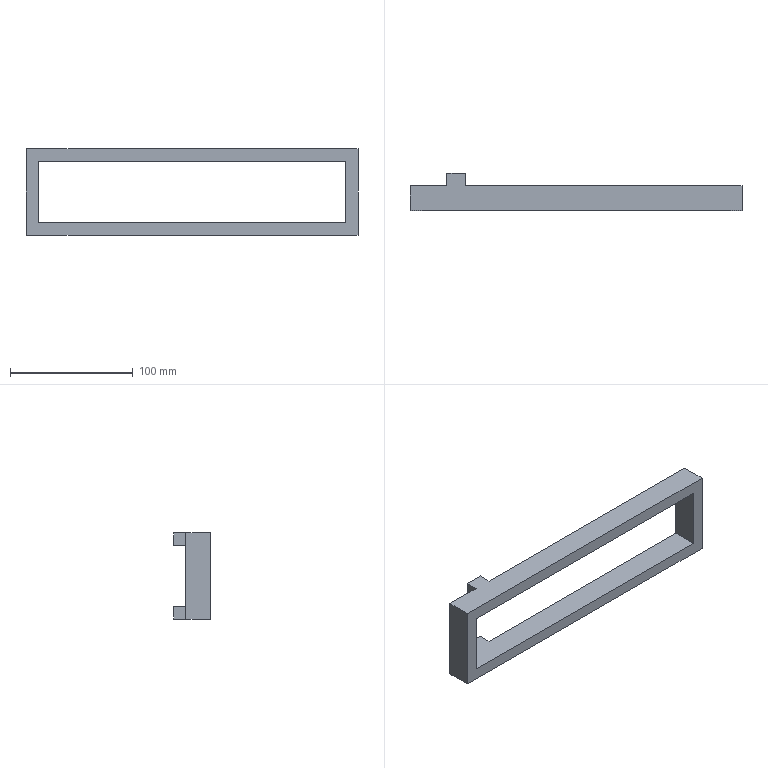Part | SolidWorks | features Extrusion 1, ICE 1, MoveFace 1 | 1 solid | 17 faces | box 270 x 30 x 70 mm | volume 131000 mm3 | plane 17
STEP:
#1=CARTESIAN_POINT('',(-120.,20.,25.));
#2=VERTEX_POINT('',#1);
#3=CARTESIAN_POINT('',(-120.,20.,35.));
#4=VERTEX_POINT('',#3);
#5=CARTESIAN_POINT('',(-120.,20.,25.));
#6=DIRECTION('',(0.,0.,1.));
#7=VECTOR('',#6,1000.);
#8=LINE('',#5,#7);
#9=EDGE_CURVE('',#2,#4,#8,.T.);
#10=ORIENTED_EDGE('',*,*,#9,.F.);
#11=CARTESIAN_POINT('',(-140.,20.,25.));
#12=VERTEX_POINT('',#11);
#13=CARTESIAN_POINT('',(-140.,20.,25.));
#14=DIRECTION('',(1.,0.,0.));
#15=VECTOR('',#14,1000.);
#16=LINE('',#13,#15);
#17=EDGE_CURVE('',#12,#2,#16,.T.);
#18=ORIENTED_EDGE('',*,*,#17,.F.);
#19=CARTESIAN_POINT('',(-140.,20.,-25.));
#20=VERTEX_POINT('',#19);
#21=CARTESIAN_POINT('',(-140.,20.,25.));
#22=DIRECTION('',(0.,0.,1.));
#23=VECTOR('',#22,1000.);
#24=LINE('',#21,#23);
#25=EDGE_CURVE('',#20,#12,#24,.T.);
#26=ORIENTED_EDGE('',*,*,#25,.F.);
#27=CARTESIAN_POINT('',(-120.,20.,-25.));
#28=VERTEX_POINT('',#27);
#29=CARTESIAN_POINT('',(-140.,20.,-25.));
#30=DIRECTION('',(-1.,0.,0.));
#31=VECTOR('',#30,1000.);
#32=LINE('',#29,#31);
#33=EDGE_CURVE('',#28,#20,#32,.T.);
#34=ORIENTED_EDGE('',*,*,#33,.F.);
#35=CARTESIAN_POINT('',(-120.,20.,-35.));
#36=VERTEX_POINT('',#35);
#37=CARTESIAN_POINT('',(-120.,20.,-35.));
#38=DIRECTION('',(0.,0.,1.));
#39=VECTOR('',#38,1000.);
#40=LINE('',#37,#39);
#41=EDGE_CURVE('',#36,#28,#40,.T.);
#42=ORIENTED_EDGE('',*,*,#41,.F.);
#43=CARTESIAN_POINT('',(-150.,20.,-35.));
#44=VERTEX_POINT('',#43);
#45=CARTESIAN_POINT('',(-150.,20.,-35.));
#46=DIRECTION('',(-1.,0.,0.));
#47=VECTOR('',#46,1000.);
#48=LINE('',#45,#47);
#49=EDGE_CURVE('',#36,#44,#48,.T.);
#50=ORIENTED_EDGE('',*,*,#49,.T.);
#51=CARTESIAN_POINT('',(-150.,20.,35.));
#52=VERTEX_POINT('',#51);
#53=CARTESIAN_POINT('',(-150.,20.,35.));
#54=DIRECTION('',(0.,0.,1.));
#55=VECTOR('',#54,1000.);
#56=LINE('',#53,#55);
#57=EDGE_CURVE('',#44,#52,#56,.T.);
#58=ORIENTED_EDGE('',*,*,#57,.T.);
#59=CARTESIAN_POINT('',(-150.,20.,35.));
#60=DIRECTION('',(1.,0.,0.));
#61=VECTOR('',#60,1000.);
#62=LINE('',#59,#61);
#63=EDGE_CURVE('',#52,#4,#62,.T.);
#64=ORIENTED_EDGE('',*,*,#63,.T.);
#65=EDGE_LOOP('',(#10,#18,#26,#34,#42,#50,#58,#64));
#66=FACE_OUTER_BOUND('',#65,.T.);
#67=CARTESIAN_POINT('',(0.,20.,0.));
#68=DIRECTION('',(0.,-1.,0.));
#69=DIRECTION('',(0.,0.,-1.));
#70=AXIS2_PLACEMENT_3D('',#67,#68,#69);
#71=PLANE('',#70);
#72=ADVANCED_FACE('',(#66),#71,.F.);
#73=CARTESIAN_POINT('',(-105.,20.,35.));
#74=VERTEX_POINT('',#73);
#75=CARTESIAN_POINT('',(-105.,20.,25.));
#76=VERTEX_POINT('',#75);
#77=CARTESIAN_POINT('',(-105.,20.,25.));
#78=DIRECTION('',(0.,0.,-1.));
#79=VECTOR('',#78,1000.);
#80=LINE('',#77,#79);
#81=EDGE_CURVE('',#74,#76,#80,.T.);
#82=ORIENTED_EDGE('',*,*,#81,.F.);
#83=CARTESIAN_POINT('',(120.,20.,35.));
#84=VERTEX_POINT('',#83);
#85=CARTESIAN_POINT('',(-150.,20.,35.));
#86=DIRECTION('',(1.,0.,0.));
#87=VECTOR('',#86,1000.);
#88=LINE('',#85,#87);
#89=EDGE_CURVE('',#74,#84,#88,.T.);
#90=ORIENTED_EDGE('',*,*,#89,.T.);
#91=CARTESIAN_POINT('',(120.,20.,-35.));
#92=VERTEX_POINT('',#91);
#93=CARTESIAN_POINT('',(120.,20.,35.));
#94=DIRECTION('',(0.,0.,-1.));
#95=VECTOR('',#94,1000.);
#96=LINE('',#93,#95);
#97=EDGE_CURVE('',#84,#92,#96,.T.);
#98=ORIENTED_EDGE('',*,*,#97,.T.);
#99=CARTESIAN_POINT('',(-105.,20.,-35.));
#100=VERTEX_POINT('',#99);
#101=CARTESIAN_POINT('',(-150.,20.,-35.));
#102=DIRECTION('',(-1.,0.,0.));
#103=VECTOR('',#102,1000.);
#104=LINE('',#101,#103);
#105=EDGE_CURVE('',#92,#100,#104,.T.);
#106=ORIENTED_EDGE('',*,*,#105,.T.);
#107=CARTESIAN_POINT('',(-105.,20.,-25.));
#108=VERTEX_POINT('',#107);
#109=CARTESIAN_POINT('',(-105.,20.,-35.));
#110=DIRECTION('',(0.,0.,-1.));
#111=VECTOR('',#110,1000.);
#112=LINE('',#109,#111);
#113=EDGE_CURVE('',#108,#100,#112,.T.);
#114=ORIENTED_EDGE('',*,*,#113,.F.);
#115=CARTESIAN_POINT('',(110.,20.,-25.));
#116=VERTEX_POINT('',#115);
#117=CARTESIAN_POINT('',(-140.,20.,-25.));
#118=DIRECTION('',(-1.,0.,0.));
#119=VECTOR('',#118,1000.);
#120=LINE('',#117,#119);
#121=EDGE_CURVE('',#116,#108,#120,.T.);
#122=ORIENTED_EDGE('',*,*,#121,.F.);
#123=CARTESIAN_POINT('',(110.,20.,25.));
#124=VERTEX_POINT('',#123);
#125=CARTESIAN_POINT('',(110.,20.,25.));
#126=DIRECTION('',(0.,0.,-1.));
#127=VECTOR('',#126,1000.);
#128=LINE('',#125,#127);
#129=EDGE_CURVE('',#124,#116,#128,.T.);
#130=ORIENTED_EDGE('',*,*,#129,.F.);
#131=CARTESIAN_POINT('',(-140.,20.,25.));
#132=DIRECTION('',(1.,0.,0.));
#133=VECTOR('',#132,1000.);
#134=LINE('',#131,#133);
#135=EDGE_CURVE('',#76,#124,#134,.T.);
#136=ORIENTED_EDGE('',*,*,#135,.F.);
#137=EDGE_LOOP('',(#82,#90,#98,#106,#114,#122,#130,#136));
#138=FACE_OUTER_BOUND('',#137,.T.);
#139=CARTESIAN_POINT('',(0.,20.,0.));
#140=DIRECTION('',(0.,-1.,0.));
#141=DIRECTION('',(0.,0.,-1.));
#142=AXIS2_PLACEMENT_3D('',#139,#140,#141);
#143=PLANE('',#142);
#144=ADVANCED_FACE('',(#138),#143,.F.);
#145=CARTESIAN_POINT('',(120.,0.,35.));
#146=VERTEX_POINT('',#145);
#147=CARTESIAN_POINT('',(120.,0.,-35.));
#148=VERTEX_POINT('',#147);
#149=CARTESIAN_POINT('',(120.,0.,35.));
#150=DIRECTION('',(0.,0.,-1.));
#151=VECTOR('',#150,1000.);
#152=LINE('',#149,#151);
#153=EDGE_CURVE('',#146,#148,#152,.T.);
#154=ORIENTED_EDGE('',*,*,#153,.F.);
#155=CARTESIAN_POINT('',(-150.,0.,35.));
#156=VERTEX_POINT('',#155);
#157=CARTESIAN_POINT('',(-150.,0.,35.));
#158=DIRECTION('',(1.,0.,0.));
#159=VECTOR('',#158,1000.);
#160=LINE('',#157,#159);
#161=EDGE_CURVE('',#156,#146,#160,.T.);
#162=ORIENTED_EDGE('',*,*,#161,.F.);
#163=CARTESIAN_POINT('',(-150.,0.,-35.));
#164=VERTEX_POINT('',#163);
#165=CARTESIAN_POINT('',(-150.,0.,35.));
#166=DIRECTION('',(0.,0.,1.));
#167=VECTOR('',#166,1000.);
#168=LINE('',#165,#167);
#169=EDGE_CURVE('',#164,#156,#168,.T.);
#170=ORIENTED_EDGE('',*,*,#169,.F.);
#171=CARTESIAN_POINT('',(-150.,0.,-35.));
#172=DIRECTION('',(-1.,0.,0.));
#173=VECTOR('',#172,1000.);
#174=LINE('',#171,#173);
#175=EDGE_CURVE('',#148,#164,#174,.T.);
#176=ORIENTED_EDGE('',*,*,#175,.F.);
#177=EDGE_LOOP('',(#154,#162,#170,#176));
#178=FACE_OUTER_BOUND('',#177,.T.);
#179=CARTESIAN_POINT('',(-140.,0.,25.));
#180=VERTEX_POINT('',#179);
#181=CARTESIAN_POINT('',(110.,0.,25.));
#182=VERTEX_POINT('',#181);
#183=CARTESIAN_POINT('',(-140.,0.,25.));
#184=DIRECTION('',(1.,0.,0.));
#185=VECTOR('',#184,1000.);
#186=LINE('',#183,#185);
#187=EDGE_CURVE('',#180,#182,#186,.T.);
#188=ORIENTED_EDGE('',*,*,#187,.T.);
#189=CARTESIAN_POINT('',(110.,0.,-25.));
#190=VERTEX_POINT('',#189);
#191=CARTESIAN_POINT('',(110.,0.,25.));
#192=DIRECTION('',(0.,0.,-1.));
#193=VECTOR('',#192,1000.);
#194=LINE('',#191,#193);
#195=EDGE_CURVE('',#182,#190,#194,.T.);
#196=ORIENTED_EDGE('',*,*,#195,.T.);
#197=CARTESIAN_POINT('',(-140.,0.,-25.));
#198=VERTEX_POINT('',#197);
#199=CARTESIAN_POINT('',(-140.,0.,-25.));
#200=DIRECTION('',(-1.,0.,0.));
#201=VECTOR('',#200,1000.);
#202=LINE('',#199,#201);
#203=EDGE_CURVE('',#190,#198,#202,.T.);
#204=ORIENTED_EDGE('',*,*,#203,.T.);
#205=CARTESIAN_POINT('',(-140.,0.,25.));
#206=DIRECTION('',(0.,0.,1.));
#207=VECTOR('',#206,1000.);
#208=LINE('',#205,#207);
#209=EDGE_CURVE('',#198,#180,#208,.T.);
#210=ORIENTED_EDGE('',*,*,#209,.T.);
#211=EDGE_LOOP('',(#188,#196,#204,#210));
#212=FACE_BOUND('',#211,.T.);
#213=CARTESIAN_POINT('',(0.,0.,0.));
#214=DIRECTION('',(0.,-1.,0.));
#215=DIRECTION('',(0.,0.,-1.));
#216=AXIS2_PLACEMENT_3D('',#213,#214,#215);
#217=PLANE('',#216);
#218=ADVANCED_FACE('',(#178,#212),#217,.T.);
#219=ORIENTED_EDGE('',*,*,#153,.T.);
#220=CARTESIAN_POINT('',(120.,20.,-35.));
#221=DIRECTION('',(0.,-1.,0.));
#222=VECTOR('',#221,1000.);
#223=LINE('',#220,#222);
#224=EDGE_CURVE('',#92,#148,#223,.T.);
#225=ORIENTED_EDGE('',*,*,#224,.F.);
#226=ORIENTED_EDGE('',*,*,#97,.F.);
#227=CARTESIAN_POINT('',(120.,20.,35.));
#228=DIRECTION('',(0.,-1.,0.));
#229=VECTOR('',#228,1000.);
#230=LINE('',#227,#229);
#231=EDGE_CURVE('',#84,#146,#230,.T.);
#232=ORIENTED_EDGE('',*,*,#231,.T.);
#233=EDGE_LOOP('',(#219,#225,#226,#232));
#234=FACE_OUTER_BOUND('',#233,.T.);
#235=CARTESIAN_POINT('',(120.,20.,35.));
#236=DIRECTION('',(-1.,0.,0.));
#237=DIRECTION('',(0.,0.,1.));
#238=AXIS2_PLACEMENT_3D('',#235,#236,#237);
#239=PLANE('',#238);
#240=ADVANCED_FACE('',(#234),#239,.F.);
#241=ORIENTED_EDGE('',*,*,#175,.T.);
#242=CARTESIAN_POINT('',(-150.,20.,-35.));
#243=DIRECTION('',(0.,-1.,0.));
#244=VECTOR('',#243,1000.);
#245=LINE('',#242,#244);
#246=EDGE_CURVE('',#44,#164,#245,.T.);
#247=ORIENTED_EDGE('',*,*,#246,.F.);
#248=ORIENTED_EDGE('',*,*,#49,.F.);
#249=CARTESIAN_POINT('',(-120.,30.,-35.));
#250=VERTEX_POINT('',#249);
#251=CARTESIAN_POINT('',(-120.,30.,-35.));
#252=DIRECTION('',(0.,-1.,0.));
#253=VECTOR('',#252,1000.);
#254=LINE('',#251,#253);
#255=EDGE_CURVE('',#250,#36,#254,.T.);
#256=ORIENTED_EDGE('',*,*,#255,.F.);
#257=CARTESIAN_POINT('',(-105.,30.,-35.));
#258=VERTEX_POINT('',#257);
#259=CARTESIAN_POINT('',(-120.,30.,-35.));
#260=DIRECTION('',(-1.,0.,0.));
#261=VECTOR('',#260,1000.);
#262=LINE('',#259,#261);
#263=EDGE_CURVE('',#258,#250,#262,.T.);
#264=ORIENTED_EDGE('',*,*,#263,.F.);
#265=CARTESIAN_POINT('',(-105.,30.,-35.));
#266=DIRECTION('',(0.,-1.,0.));
#267=VECTOR('',#266,1000.);
#268=LINE('',#265,#267);
#269=EDGE_CURVE('',#258,#100,#268,.T.);
#270=ORIENTED_EDGE('',*,*,#269,.T.);
#271=ORIENTED_EDGE('',*,*,#105,.F.);
#272=ORIENTED_EDGE('',*,*,#224,.T.);
#273=EDGE_LOOP('',(#241,#247,#248,#256,#264,#270,#271,#272));
#274=FACE_OUTER_BOUND('',#273,.T.);
#275=CARTESIAN_POINT('',(-150.,20.,-35.));
#276=DIRECTION('',(0.,0.,1.));
#277=DIRECTION('',(1.,0.,0.));
#278=AXIS2_PLACEMENT_3D('',#275,#276,#277);
#279=PLANE('',#278);
#280=ADVANCED_FACE('',(#274),#279,.F.);
#281=ORIENTED_EDGE('',*,*,#169,.T.);
#282=CARTESIAN_POINT('',(-150.,20.,35.));
#283=DIRECTION('',(0.,-1.,0.));
#284=VECTOR('',#283,1000.);
#285=LINE('',#282,#284);
#286=EDGE_CURVE('',#52,#156,#285,.T.);
#287=ORIENTED_EDGE('',*,*,#286,.F.);
#288=ORIENTED_EDGE('',*,*,#57,.F.);
#289=ORIENTED_EDGE('',*,*,#246,.T.);
#290=EDGE_LOOP('',(#281,#287,#288,#289));
#291=FACE_OUTER_BOUND('',#290,.T.);
#292=CARTESIAN_POINT('',(-150.,20.,35.));
#293=DIRECTION('',(1.,0.,0.));
#294=DIRECTION('',(0.,0.,-1.));
#295=AXIS2_PLACEMENT_3D('',#292,#293,#294);
#296=PLANE('',#295);
#297=ADVANCED_FACE('',(#291),#296,.F.);
#298=ORIENTED_EDGE('',*,*,#161,.T.);
#299=ORIENTED_EDGE('',*,*,#231,.F.);
#300=ORIENTED_EDGE('',*,*,#89,.F.);
#301=CARTESIAN_POINT('',(-105.,30.,35.));
#302=VERTEX_POINT('',#301);
#303=CARTESIAN_POINT('',(-105.,30.,35.));
#304=DIRECTION('',(0.,-1.,0.));
#305=VECTOR('',#304,1000.);
#306=LINE('',#303,#305);
#307=EDGE_CURVE('',#302,#74,#306,.T.);
#308=ORIENTED_EDGE('',*,*,#307,.F.);
#309=CARTESIAN_POINT('',(-120.,30.,35.));
#310=VERTEX_POINT('',#309);
#311=CARTESIAN_POINT('',(-120.,30.,35.));
#312=DIRECTION('',(1.,0.,0.));
#313=VECTOR('',#312,1000.);
#314=LINE('',#311,#313);
#315=EDGE_CURVE('',#310,#302,#314,.T.);
#316=ORIENTED_EDGE('',*,*,#315,.F.);
#317=CARTESIAN_POINT('',(-120.,30.,35.));
#318=DIRECTION('',(0.,-1.,0.));
#319=VECTOR('',#318,1000.);
#320=LINE('',#317,#319);
#321=EDGE_CURVE('',#310,#4,#320,.T.);
#322=ORIENTED_EDGE('',*,*,#321,.T.);
#323=ORIENTED_EDGE('',*,*,#63,.F.);
#324=ORIENTED_EDGE('',*,*,#286,.T.);
#325=EDGE_LOOP('',(#298,#299,#300,#308,#316,#322,#323,#324));
#326=FACE_OUTER_BOUND('',#325,.T.);
#327=CARTESIAN_POINT('',(-150.,20.,35.));
#328=DIRECTION('',(0.,0.,-1.));
#329=DIRECTION('',(-1.,0.,0.));
#330=AXIS2_PLACEMENT_3D('',#327,#328,#329);
#331=PLANE('',#330);
#332=ADVANCED_FACE('',(#326),#331,.F.);
#333=ORIENTED_EDGE('',*,*,#195,.F.);
#334=CARTESIAN_POINT('',(110.,20.,25.));
#335=DIRECTION('',(0.,-1.,0.));
#336=VECTOR('',#335,1000.);
#337=LINE('',#334,#336);
#338=EDGE_CURVE('',#124,#182,#337,.T.);
#339=ORIENTED_EDGE('',*,*,#338,.F.);
#340=ORIENTED_EDGE('',*,*,#129,.T.);
#341=CARTESIAN_POINT('',(110.,20.,-25.));
#342=DIRECTION('',(0.,-1.,0.));
#343=VECTOR('',#342,1000.);
#344=LINE('',#341,#343);
#345=EDGE_CURVE('',#116,#190,#344,.T.);
#346=ORIENTED_EDGE('',*,*,#345,.T.);
#347=EDGE_LOOP('',(#333,#339,#340,#346));
#348=FACE_OUTER_BOUND('',#347,.T.);
#349=CARTESIAN_POINT('',(110.,20.,25.));
#350=DIRECTION('',(-1.,0.,0.));
#351=DIRECTION('',(0.,0.,1.));
#352=AXIS2_PLACEMENT_3D('',#349,#350,#351);
#353=PLANE('',#352);
#354=ADVANCED_FACE('',(#348),#353,.T.);
#355=ORIENTED_EDGE('',*,*,#203,.F.);
#356=ORIENTED_EDGE('',*,*,#345,.F.);
#357=ORIENTED_EDGE('',*,*,#121,.T.);
#358=CARTESIAN_POINT('',(-105.,30.,-25.));
#359=VERTEX_POINT('',#358);
#360=CARTESIAN_POINT('',(-105.,30.,-25.));
#361=DIRECTION('',(0.,-1.,0.));
#362=VECTOR('',#361,1000.);
#363=LINE('',#360,#362);
#364=EDGE_CURVE('',#359,#108,#363,.T.);
#365=ORIENTED_EDGE('',*,*,#364,.F.);
#366=CARTESIAN_POINT('',(-120.,30.,-25.));
#367=VERTEX_POINT('',#366);
#368=CARTESIAN_POINT('',(-120.,30.,-25.));
#369=DIRECTION('',(1.,0.,0.));
#370=VECTOR('',#369,1000.);
#371=LINE('',#368,#370);
#372=EDGE_CURVE('',#367,#359,#371,.T.);
#373=ORIENTED_EDGE('',*,*,#372,.F.);
#374=CARTESIAN_POINT('',(-120.,30.,-25.));
#375=DIRECTION('',(0.,-1.,0.));
#376=VECTOR('',#375,1000.);
#377=LINE('',#374,#376);
#378=EDGE_CURVE('',#367,#28,#377,.T.);
#379=ORIENTED_EDGE('',*,*,#378,.T.);
#380=ORIENTED_EDGE('',*,*,#33,.T.);
#381=CARTESIAN_POINT('',(-140.,20.,-25.));
#382=DIRECTION('',(0.,-1.,0.));
#383=VECTOR('',#382,1000.);
#384=LINE('',#381,#383);
#385=EDGE_CURVE('',#20,#198,#384,.T.);
#386=ORIENTED_EDGE('',*,*,#385,.T.);
#387=EDGE_LOOP('',(#355,#356,#357,#365,#373,#379,#380,#386));
#388=FACE_OUTER_BOUND('',#387,.T.);
#389=CARTESIAN_POINT('',(-140.,20.,-25.));
#390=DIRECTION('',(0.,0.,1.));
#391=DIRECTION('',(1.,0.,0.));
#392=AXIS2_PLACEMENT_3D('',#389,#390,#391);
#393=PLANE('',#392);
#394=ADVANCED_FACE('',(#388),#393,.T.);
#395=ORIENTED_EDGE('',*,*,#209,.F.);
#396=ORIENTED_EDGE('',*,*,#385,.F.);
#397=ORIENTED_EDGE('',*,*,#25,.T.);
#398=CARTESIAN_POINT('',(-140.,20.,25.));
#399=DIRECTION('',(0.,-1.,0.));
#400=VECTOR('',#399,1000.);
#401=LINE('',#398,#400);
#402=EDGE_CURVE('',#12,#180,#401,.T.);
#403=ORIENTED_EDGE('',*,*,#402,.T.);
#404=EDGE_LOOP('',(#395,#396,#397,#403));
#405=FACE_OUTER_BOUND('',#404,.T.);
#406=CARTESIAN_POINT('',(-140.,20.,25.));
#407=DIRECTION('',(1.,0.,0.));
#408=DIRECTION('',(0.,0.,-1.));
#409=AXIS2_PLACEMENT_3D('',#406,#407,#408);
#410=PLANE('',#409);
#411=ADVANCED_FACE('',(#405),#410,.T.);
#412=ORIENTED_EDGE('',*,*,#187,.F.);
#413=ORIENTED_EDGE('',*,*,#402,.F.);
#414=ORIENTED_EDGE('',*,*,#17,.T.);
#415=CARTESIAN_POINT('',(-120.,30.,25.));
#416=VERTEX_POINT('',#415);
#417=CARTESIAN_POINT('',(-120.,30.,25.));
#418=DIRECTION('',(0.,-1.,0.));
#419=VECTOR('',#418,1000.);
#420=LINE('',#417,#419);
#421=EDGE_CURVE('',#416,#2,#420,.T.);
#422=ORIENTED_EDGE('',*,*,#421,.F.);
#423=CARTESIAN_POINT('',(-105.,30.,25.));
#424=VERTEX_POINT('',#423);
#425=CARTESIAN_POINT('',(-120.,30.,25.));
#426=DIRECTION('',(-1.,0.,0.));
#427=VECTOR('',#426,1000.);
#428=LINE('',#425,#427);
#429=EDGE_CURVE('',#424,#416,#428,.T.);
#430=ORIENTED_EDGE('',*,*,#429,.F.);
#431=CARTESIAN_POINT('',(-105.,30.,25.));
#432=DIRECTION('',(0.,-1.,0.));
#433=VECTOR('',#432,1000.);
#434=LINE('',#431,#433);
#435=EDGE_CURVE('',#424,#76,#434,.T.);
#436=ORIENTED_EDGE('',*,*,#435,.T.);
#437=ORIENTED_EDGE('',*,*,#135,.T.);
#438=ORIENTED_EDGE('',*,*,#338,.T.);
#439=EDGE_LOOP('',(#412,#413,#414,#422,#430,#436,#437,#438));
#440=FACE_OUTER_BOUND('',#439,.T.);
#441=CARTESIAN_POINT('',(-140.,20.,25.));
#442=DIRECTION('',(0.,0.,-1.));
#443=DIRECTION('',(-1.,0.,0.));
#444=AXIS2_PLACEMENT_3D('',#441,#442,#443);
#445=PLANE('',#444);
#446=ADVANCED_FACE('',(#440),#445,.T.);
#447=ORIENTED_EDGE('',*,*,#41,.T.);
#448=ORIENTED_EDGE('',*,*,#378,.F.);
#449=CARTESIAN_POINT('',(-120.,30.,-35.));
#450=DIRECTION('',(0.,0.,1.));
#451=VECTOR('',#450,1000.);
#452=LINE('',#449,#451);
#453=EDGE_CURVE('',#250,#367,#452,.T.);
#454=ORIENTED_EDGE('',*,*,#453,.F.);
#455=ORIENTED_EDGE('',*,*,#255,.T.);
#456=EDGE_LOOP('',(#447,#448,#454,#455));
#457=FACE_OUTER_BOUND('',#456,.T.);
#458=CARTESIAN_POINT('',(-120.,30.,-35.));
#459=DIRECTION('',(1.,0.,0.));
#460=DIRECTION('',(0.,0.,-1.));
#461=AXIS2_PLACEMENT_3D('',#458,#459,#460);
#462=PLANE('',#461);
#463=ADVANCED_FACE('',(#457),#462,.F.);
#464=ORIENTED_EDGE('',*,*,#113,.T.);
#465=ORIENTED_EDGE('',*,*,#269,.F.);
#466=CARTESIAN_POINT('',(-105.,30.,-35.));
#467=DIRECTION('',(0.,0.,-1.));
#468=VECTOR('',#467,1000.);
#469=LINE('',#466,#468);
#470=EDGE_CURVE('',#359,#258,#469,.T.);
#471=ORIENTED_EDGE('',*,*,#470,.F.);
#472=ORIENTED_EDGE('',*,*,#364,.T.);
#473=EDGE_LOOP('',(#464,#465,#471,#472));
#474=FACE_OUTER_BOUND('',#473,.T.);
#475=CARTESIAN_POINT('',(-105.,30.,-35.));
#476=DIRECTION('',(-1.,0.,0.));
#477=DIRECTION('',(0.,0.,1.));
#478=AXIS2_PLACEMENT_3D('',#475,#476,#477);
#479=PLANE('',#478);
#480=ADVANCED_FACE('',(#474),#479,.F.);
#481=ORIENTED_EDGE('',*,*,#453,.T.);
#482=ORIENTED_EDGE('',*,*,#372,.T.);
#483=ORIENTED_EDGE('',*,*,#470,.T.);
#484=ORIENTED_EDGE('',*,*,#263,.T.);
#485=EDGE_LOOP('',(#481,#482,#483,#484));
#486=FACE_OUTER_BOUND('',#485,.T.);
#487=CARTESIAN_POINT('',(0.,30.,0.));
#488=DIRECTION('',(0.,1.,0.));
#489=DIRECTION('',(0.,0.,1.));
#490=AXIS2_PLACEMENT_3D('',#487,#488,#489);
#491=PLANE('',#490);
#492=ADVANCED_FACE('',(#486),#491,.T.);
#493=ORIENTED_EDGE('',*,*,#9,.T.);
#494=ORIENTED_EDGE('',*,*,#321,.F.);
#495=CARTESIAN_POINT('',(-120.,30.,25.));
#496=DIRECTION('',(0.,0.,1.));
#497=VECTOR('',#496,1000.);
#498=LINE('',#495,#497);
#499=EDGE_CURVE('',#416,#310,#498,.T.);
#500=ORIENTED_EDGE('',*,*,#499,.F.);
#501=ORIENTED_EDGE('',*,*,#421,.T.);
#502=EDGE_LOOP('',(#493,#494,#500,#501));
#503=FACE_OUTER_BOUND('',#502,.T.);
#504=CARTESIAN_POINT('',(-120.,30.,25.));
#505=DIRECTION('',(1.,0.,0.));
#506=DIRECTION('',(0.,0.,-1.));
#507=AXIS2_PLACEMENT_3D('',#504,#505,#506);
#508=PLANE('',#507);
#509=ADVANCED_FACE('',(#503),#508,.F.);
#510=ORIENTED_EDGE('',*,*,#81,.T.);
#511=ORIENTED_EDGE('',*,*,#435,.F.);
#512=CARTESIAN_POINT('',(-105.,30.,25.));
#513=DIRECTION('',(0.,0.,-1.));
#514=VECTOR('',#513,1000.);
#515=LINE('',#512,#514);
#516=EDGE_CURVE('',#302,#424,#515,.T.);
#517=ORIENTED_EDGE('',*,*,#516,.F.);
#518=ORIENTED_EDGE('',*,*,#307,.T.);
#519=EDGE_LOOP('',(#510,#511,#517,#518));
#520=FACE_OUTER_BOUND('',#519,.T.);
#521=CARTESIAN_POINT('',(-105.,30.,25.));
#522=DIRECTION('',(-1.,0.,0.));
#523=DIRECTION('',(0.,0.,1.));
#524=AXIS2_PLACEMENT_3D('',#521,#522,#523);
#525=PLANE('',#524);
#526=ADVANCED_FACE('',(#520),#525,.F.);
#527=ORIENTED_EDGE('',*,*,#499,.T.);
#528=ORIENTED_EDGE('',*,*,#315,.T.);
#529=ORIENTED_EDGE('',*,*,#516,.T.);
#530=ORIENTED_EDGE('',*,*,#429,.T.);
#531=EDGE_LOOP('',(#527,#528,#529,#530));
#532=FACE_OUTER_BOUND('',#531,.T.);
#533=CARTESIAN_POINT('',(0.,30.,0.));
#534=DIRECTION('',(0.,1.,0.));
#535=DIRECTION('',(0.,0.,1.));
#536=AXIS2_PLACEMENT_3D('',#533,#534,#535);
#537=PLANE('',#536);
#538=ADVANCED_FACE('',(#532),#537,.T.);
#539=CLOSED_SHELL('',(#72,#144,#218,#240,#280,#297,#332,#354,#394,#411,#446,#463,#480,#492,#509,#526,#538));
#540=MANIFOLD_SOLID_BREP('',#539);
#541=CARTESIAN_POINT('',(0.,0.,0.));
#542=DIRECTION('',(0.,0.,1.));
#543=DIRECTION('',(1.,0.,0.));
#544=AXIS2_PLACEMENT_3D('',#541,#542,#543);
#545=(LENGTH_UNIT()NAMED_UNIT(*)SI_UNIT(.MILLI.,.METRE.));
#546=UNCERTAINTY_MEASURE_WITH_UNIT(LENGTH_MEASURE(0.00001),#545,'','');
#547=(NAMED_UNIT(*)PLANE_ANGLE_UNIT()SI_UNIT($,.RADIAN.));
#548=(NAMED_UNIT(*)SI_UNIT($,.STERADIAN.)SOLID_ANGLE_UNIT());
#549=(GEOMETRIC_REPRESENTATION_CONTEXT(3)GLOBAL_UNCERTAINTY_ASSIGNED_CONTEXT((#546))GLOBAL_UNIT_ASSIGNED_CONTEXT((#545,#547,#548))REPRESENTATION_CONTEXT('',''));
#550=ADVANCED_BREP_SHAPE_REPRESENTATION('',(#540,#544),#549);